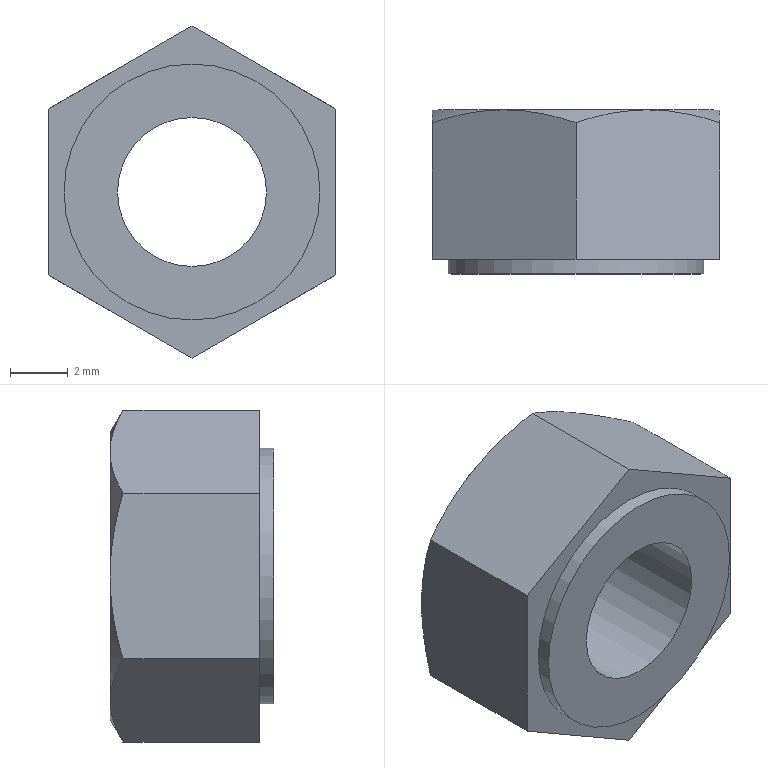Part | STEP file | Tube necking machine_id202_x_t | 1 solid | 18 faces | box 10 x 5.7 x 11.547 mm | volume 357.493 mm3 | plane 9 | cone 7 | cylinder 2 | commonest cylinder face diameters 5.188 x1 8.9 x1